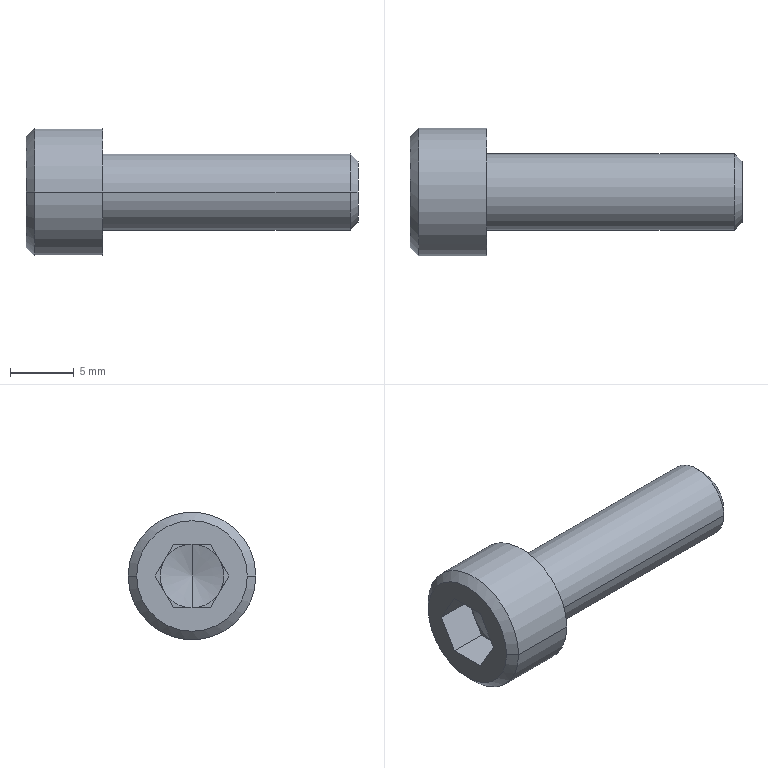Part | STEP file | CB6-20_デフォルト | 1 solid | 25 faces | box 26 x 10 x 10 mm | volume 957.413 mm3 | plane 15 | cone 6 | cylinder 4 | commonest cylinder face diameters 6 x2 10 x2